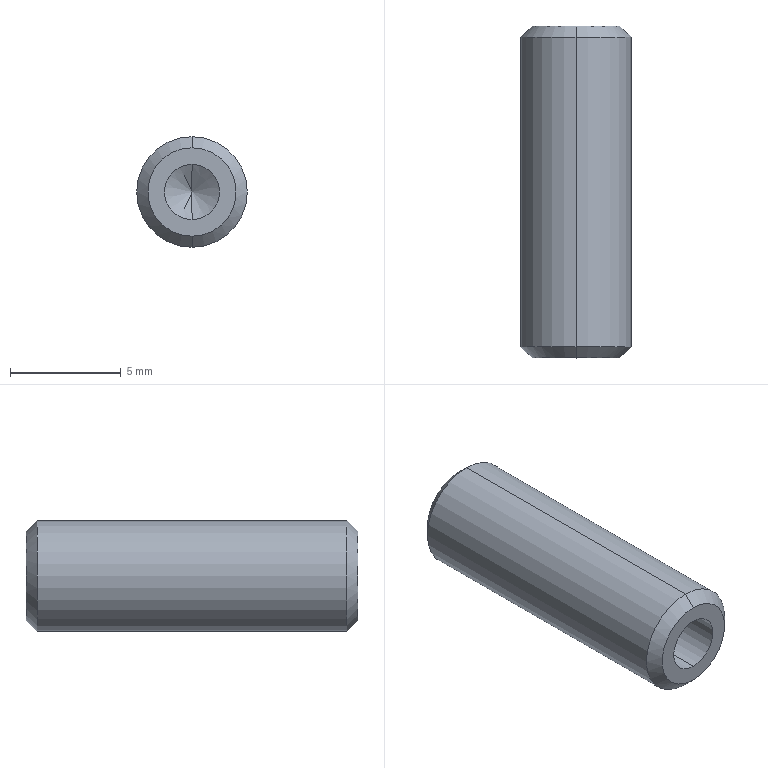Part | SolidWorks | features Chamfer 1, Extrusion 1, HoleWzd 1 | 1 solid | 12 faces | box 5 x 15 x 5 mm | volume 252.815 mm3 | cone 6 | cylinder 4 | plane 2 | commonest cylinder face diameters 2.5 x2 5 x2
STEP:
#1=CARTESIAN_POINT('',(0.,15.,2.));
#2=VERTEX_POINT('',#1);
#3=CARTESIAN_POINT('',(0.,15.,-2.));
#4=VERTEX_POINT('',#3);
#5=CARTESIAN_POINT('',(0.,15.,0.));
#6=DIRECTION('',(0.,1.,0.));
#7=DIRECTION('',(0.,0.,1.));
#8=AXIS2_PLACEMENT_3D('',#5,#6,#7);
#9=CIRCLE('',#8,2.);
#10=EDGE_CURVE('',#2,#4,#9,.T.);
#11=ORIENTED_EDGE('',*,*,#10,.F.);
#12=CARTESIAN_POINT('',(0.,14.5,2.5));
#13=VERTEX_POINT('',#12);
#14=CARTESIAN_POINT('',(0.,15.,2.));
#15=DIRECTION('',(0.,-0.7071,0.7071));
#16=VECTOR('',#15,1000.);
#17=LINE('',#14,#16);
#18=EDGE_CURVE('',#2,#13,#17,.T.);
#19=ORIENTED_EDGE('',*,*,#18,.T.);
#20=CARTESIAN_POINT('',(0.,14.5,-2.5));
#21=VERTEX_POINT('',#20);
#22=CARTESIAN_POINT('',(0.,14.5,0.));
#23=DIRECTION('',(0.,-1.,0.));
#24=DIRECTION('',(0.,0.,1.));
#25=AXIS2_PLACEMENT_3D('',#22,#23,#24);
#26=CIRCLE('',#25,2.5);
#27=EDGE_CURVE('',#21,#13,#26,.T.);
#28=ORIENTED_EDGE('',*,*,#27,.F.);
#29=CARTESIAN_POINT('',(0.,15.,-2.));
#30=DIRECTION('',(0.,-0.7071,-0.7071));
#31=VECTOR('',#30,1000.);
#32=LINE('',#29,#31);
#33=EDGE_CURVE('',#4,#21,#32,.T.);
#34=ORIENTED_EDGE('',*,*,#33,.F.);
#35=EDGE_LOOP('',(#11,#19,#28,#34));
#36=FACE_OUTER_BOUND('',#35,.T.);
#37=CARTESIAN_POINT('',(0.,15.,0.));
#38=DIRECTION('',(0.,-1.,0.));
#39=DIRECTION('',(0.,0.,-1.));
#40=AXIS2_PLACEMENT_3D('',#37,#38,#39);
#41=CONICAL_SURFACE('',#40,2.,0.7854);
#42=ADVANCED_FACE('',(#36),#41,.T.);
#43=CARTESIAN_POINT('',(0.,0.,-2.));
#44=VERTEX_POINT('',#43);
#45=CARTESIAN_POINT('',(0.,0.,2.));
#46=VERTEX_POINT('',#45);
#47=CARTESIAN_POINT('',(0.,0.,0.));
#48=DIRECTION('',(0.,-1.,0.));
#49=DIRECTION('',(0.,0.,1.));
#50=AXIS2_PLACEMENT_3D('',#47,#48,#49);
#51=CIRCLE('',#50,2.);
#52=EDGE_CURVE('',#44,#46,#51,.T.);
#53=ORIENTED_EDGE('',*,*,#52,.F.);
#54=CARTESIAN_POINT('',(0.,0.5,-2.5));
#55=VERTEX_POINT('',#54);
#56=CARTESIAN_POINT('',(0.,0.5,-2.5));
#57=DIRECTION('',(0.,0.7071,-0.7071));
#58=VECTOR('',#57,1000.);
#59=LINE('',#56,#58);
#60=EDGE_CURVE('',#44,#55,#59,.T.);
#61=ORIENTED_EDGE('',*,*,#60,.T.);
#62=CARTESIAN_POINT('',(0.,0.5,2.5));
#63=VERTEX_POINT('',#62);
#64=CARTESIAN_POINT('',(0.,0.5,0.));
#65=DIRECTION('',(0.,1.,0.));
#66=DIRECTION('',(0.,0.,1.));
#67=AXIS2_PLACEMENT_3D('',#64,#65,#66);
#68=CIRCLE('',#67,2.5);
#69=EDGE_CURVE('',#63,#55,#68,.T.);
#70=ORIENTED_EDGE('',*,*,#69,.F.);
#71=CARTESIAN_POINT('',(0.,0.5,2.5));
#72=DIRECTION('',(0.,0.7071,0.7071));
#73=VECTOR('',#72,1000.);
#74=LINE('',#71,#73);
#75=EDGE_CURVE('',#46,#63,#74,.T.);
#76=ORIENTED_EDGE('',*,*,#75,.F.);
#77=EDGE_LOOP('',(#53,#61,#70,#76));
#78=FACE_OUTER_BOUND('',#77,.T.);
#79=CARTESIAN_POINT('',(0.,0.5,0.));
#80=DIRECTION('',(0.,1.,0.));
#81=DIRECTION('',(0.,0.,1.));
#82=AXIS2_PLACEMENT_3D('',#79,#80,#81);
#83=CONICAL_SURFACE('',#82,2.5,0.7854);
#84=ADVANCED_FACE('',(#78),#83,.T.);
#85=CARTESIAN_POINT('',(0.,7.5,1.25));
#86=VERTEX_POINT('',#85);
#87=CARTESIAN_POINT('',(0.,7.5,-1.25));
#88=VERTEX_POINT('',#87);
#89=CARTESIAN_POINT('',(0.,7.5,0.));
#90=DIRECTION('',(0.,-1.,0.));
#91=DIRECTION('',(0.,0.,-1.));
#92=AXIS2_PLACEMENT_3D('',#89,#90,#91);
#93=CIRCLE('',#92,1.25);
#94=EDGE_CURVE('',#86,#88,#93,.T.);
#95=ORIENTED_EDGE('',*,*,#94,.F.);
#96=CARTESIAN_POINT('',(0.,0.,1.25));
#97=VERTEX_POINT('',#96);
#98=CARTESIAN_POINT('',(0.,0.,1.25));
#99=DIRECTION('',(0.,-1.,0.));
#100=VECTOR('',#99,1000.);
#101=LINE('',#98,#100);
#102=EDGE_CURVE('',#86,#97,#101,.T.);
#103=ORIENTED_EDGE('',*,*,#102,.T.);
#104=CARTESIAN_POINT('',(0.,0.,-1.25));
#105=VERTEX_POINT('',#104);
#106=CARTESIAN_POINT('',(0.,0.,0.));
#107=DIRECTION('',(0.,-1.,0.));
#108=DIRECTION('',(0.,0.,-1.));
#109=AXIS2_PLACEMENT_3D('',#106,#107,#108);
#110=CIRCLE('',#109,1.25);
#111=EDGE_CURVE('',#97,#105,#110,.T.);
#112=ORIENTED_EDGE('',*,*,#111,.T.);
#113=CARTESIAN_POINT('',(0.,0.,-1.25));
#114=DIRECTION('',(0.,-1.,0.));
#115=VECTOR('',#114,1000.);
#116=LINE('',#113,#115);
#117=EDGE_CURVE('',#88,#105,#116,.T.);
#118=ORIENTED_EDGE('',*,*,#117,.F.);
#119=EDGE_LOOP('',(#95,#103,#112,#118));
#120=FACE_OUTER_BOUND('',#119,.T.);
#121=CARTESIAN_POINT('',(0.,0.,0.));
#122=DIRECTION('',(0.,-1.,0.));
#123=DIRECTION('',(0.,0.,-1.));
#124=AXIS2_PLACEMENT_3D('',#121,#122,#123);
#125=CYLINDRICAL_SURFACE('',#124,1.25);
#126=ADVANCED_FACE('',(#120),#125,.F.);
#127=CARTESIAN_POINT('',(0.,8.251,0.));
#128=VERTEX_POINT('',#127);
#129=CARTESIAN_POINT('',(0.,7.5,-1.25));
#130=DIRECTION('',(0.,-0.515,-0.8572));
#131=VECTOR('',#130,1000.);
#132=LINE('',#129,#131);
#133=EDGE_CURVE('',#128,#88,#132,.T.);
#134=ORIENTED_EDGE('',*,*,#133,.F.);
#135=CARTESIAN_POINT('',(0.,7.5,1.25));
#136=DIRECTION('',(0.,-0.515,0.8572));
#137=VECTOR('',#136,1000.);
#138=LINE('',#135,#137);
#139=EDGE_CURVE('',#128,#86,#138,.T.);
#140=ORIENTED_EDGE('',*,*,#139,.T.);
#141=ORIENTED_EDGE('',*,*,#94,.T.);
#142=EDGE_LOOP('',(#134,#140,#141));
#143=FACE_OUTER_BOUND('',#142,.T.);
#144=CARTESIAN_POINT('',(0.,7.5,0.));
#145=DIRECTION('',(0.,-1.,0.));
#146=DIRECTION('',(0.,0.,-1.));
#147=AXIS2_PLACEMENT_3D('',#144,#145,#146);
#148=CONICAL_SURFACE('',#147,1.25,1.03);
#149=ADVANCED_FACE('',(#143),#148,.F.);
#150=ORIENTED_EDGE('',*,*,#27,.T.);
#151=CARTESIAN_POINT('',(0.,15.,2.5));
#152=DIRECTION('',(0.,-1.,0.));
#153=VECTOR('',#152,1000.);
#154=LINE('',#151,#153);
#155=EDGE_CURVE('',#13,#63,#154,.T.);
#156=ORIENTED_EDGE('',*,*,#155,.T.);
#157=ORIENTED_EDGE('',*,*,#69,.T.);
#158=CARTESIAN_POINT('',(0.,15.,-2.5));
#159=DIRECTION('',(0.,-1.,0.));
#160=VECTOR('',#159,1000.);
#161=LINE('',#158,#160);
#162=EDGE_CURVE('',#21,#55,#161,.T.);
#163=ORIENTED_EDGE('',*,*,#162,.F.);
#164=EDGE_LOOP('',(#150,#156,#157,#163));
#165=FACE_OUTER_BOUND('',#164,.T.);
#166=CARTESIAN_POINT('',(0.,15.,0.));
#167=DIRECTION('',(0.,-1.,0.));
#168=DIRECTION('',(0.,0.,-1.));
#169=AXIS2_PLACEMENT_3D('',#166,#167,#168);
#170=CYLINDRICAL_SURFACE('',#169,2.5);
#171=ADVANCED_FACE('',(#165),#170,.T.);
#172=ORIENTED_EDGE('',*,*,#155,.F.);
#173=CARTESIAN_POINT('',(0.,14.5,0.));
#174=DIRECTION('',(0.,-1.,0.));
#175=DIRECTION('',(0.,0.,1.));
#176=AXIS2_PLACEMENT_3D('',#173,#174,#175);
#177=CIRCLE('',#176,2.5);
#178=EDGE_CURVE('',#13,#21,#177,.T.);
#179=ORIENTED_EDGE('',*,*,#178,.T.);
#180=ORIENTED_EDGE('',*,*,#162,.T.);
#181=CARTESIAN_POINT('',(0.,0.5,0.));
#182=DIRECTION('',(0.,1.,0.));
#183=DIRECTION('',(0.,0.,1.));
#184=AXIS2_PLACEMENT_3D('',#181,#182,#183);
#185=CIRCLE('',#184,2.5);
#186=EDGE_CURVE('',#55,#63,#185,.T.);
#187=ORIENTED_EDGE('',*,*,#186,.T.);
#188=EDGE_LOOP('',(#172,#179,#180,#187));
#189=FACE_OUTER_BOUND('',#188,.T.);
#190=CARTESIAN_POINT('',(0.,15.,0.));
#191=DIRECTION('',(0.,-1.,0.));
#192=DIRECTION('',(0.,0.,-1.));
#193=AXIS2_PLACEMENT_3D('',#190,#191,#192);
#194=CYLINDRICAL_SURFACE('',#193,2.5);
#195=ADVANCED_FACE('',(#189),#194,.T.);
#196=CARTESIAN_POINT('',(0.,15.,0.));
#197=DIRECTION('',(0.,1.,0.));
#198=DIRECTION('',(0.,0.,1.));
#199=AXIS2_PLACEMENT_3D('',#196,#197,#198);
#200=CIRCLE('',#199,2.);
#201=EDGE_CURVE('',#4,#2,#200,.T.);
#202=ORIENTED_EDGE('',*,*,#201,.T.);
#203=ORIENTED_EDGE('',*,*,#10,.T.);
#204=EDGE_LOOP('',(#202,#203));
#205=FACE_OUTER_BOUND('',#204,.T.);
#206=CARTESIAN_POINT('',(0.,15.,0.));
#207=DIRECTION('',(0.,1.,0.));
#208=DIRECTION('',(0.,0.,1.));
#209=AXIS2_PLACEMENT_3D('',#206,#207,#208);
#210=PLANE('',#209);
#211=ADVANCED_FACE('',(#205),#210,.T.);
#212=CARTESIAN_POINT('',(0.,0.,0.));
#213=DIRECTION('',(0.,-1.,0.));
#214=DIRECTION('',(0.,0.,1.));
#215=AXIS2_PLACEMENT_3D('',#212,#213,#214);
#216=CIRCLE('',#215,2.);
#217=EDGE_CURVE('',#46,#44,#216,.T.);
#218=ORIENTED_EDGE('',*,*,#217,.T.);
#219=ORIENTED_EDGE('',*,*,#52,.T.);
#220=EDGE_LOOP('',(#218,#219));
#221=FACE_OUTER_BOUND('',#220,.T.);
#222=CARTESIAN_POINT('',(0.,0.,0.));
#223=DIRECTION('',(0.,-1.,0.));
#224=DIRECTION('',(0.,0.,-1.));
#225=AXIS2_PLACEMENT_3D('',#222,#223,#224);
#226=CIRCLE('',#225,1.25);
#227=EDGE_CURVE('',#105,#97,#226,.T.);
#228=ORIENTED_EDGE('',*,*,#227,.F.);
#229=ORIENTED_EDGE('',*,*,#111,.F.);
#230=EDGE_LOOP('',(#228,#229));
#231=FACE_BOUND('',#230,.T.);
#232=CARTESIAN_POINT('',(0.,0.,0.));
#233=DIRECTION('',(0.,1.,0.));
#234=DIRECTION('',(0.,0.,1.));
#235=AXIS2_PLACEMENT_3D('',#232,#233,#234);
#236=PLANE('',#235);
#237=ADVANCED_FACE('',(#221,#231),#236,.F.);
#238=ORIENTED_EDGE('',*,*,#139,.F.);
#239=ORIENTED_EDGE('',*,*,#133,.T.);
#240=CARTESIAN_POINT('',(0.,7.5,0.));
#241=DIRECTION('',(0.,-1.,0.));
#242=DIRECTION('',(0.,0.,-1.));
#243=AXIS2_PLACEMENT_3D('',#240,#241,#242);
#244=CIRCLE('',#243,1.25);
#245=EDGE_CURVE('',#88,#86,#244,.T.);
#246=ORIENTED_EDGE('',*,*,#245,.T.);
#247=EDGE_LOOP('',(#238,#239,#246));
#248=FACE_OUTER_BOUND('',#247,.T.);
#249=CARTESIAN_POINT('',(0.,7.5,0.));
#250=DIRECTION('',(0.,-1.,0.));
#251=DIRECTION('',(0.,0.,-1.));
#252=AXIS2_PLACEMENT_3D('',#249,#250,#251);
#253=CONICAL_SURFACE('',#252,1.25,1.03);
#254=ADVANCED_FACE('',(#248),#253,.F.);
#255=ORIENTED_EDGE('',*,*,#102,.F.);
#256=ORIENTED_EDGE('',*,*,#245,.F.);
#257=ORIENTED_EDGE('',*,*,#117,.T.);
#258=ORIENTED_EDGE('',*,*,#227,.T.);
#259=EDGE_LOOP('',(#255,#256,#257,#258));
#260=FACE_OUTER_BOUND('',#259,.T.);
#261=CARTESIAN_POINT('',(0.,0.,0.));
#262=DIRECTION('',(0.,-1.,0.));
#263=DIRECTION('',(0.,0.,-1.));
#264=AXIS2_PLACEMENT_3D('',#261,#262,#263);
#265=CYLINDRICAL_SURFACE('',#264,1.25);
#266=ADVANCED_FACE('',(#260),#265,.F.);
#267=ORIENTED_EDGE('',*,*,#60,.F.);
#268=ORIENTED_EDGE('',*,*,#217,.F.);
#269=ORIENTED_EDGE('',*,*,#75,.T.);
#270=ORIENTED_EDGE('',*,*,#186,.F.);
#271=EDGE_LOOP('',(#267,#268,#269,#270));
#272=FACE_OUTER_BOUND('',#271,.T.);
#273=CARTESIAN_POINT('',(0.,0.5,0.));
#274=DIRECTION('',(0.,1.,0.));
#275=DIRECTION('',(0.,0.,1.));
#276=AXIS2_PLACEMENT_3D('',#273,#274,#275);
#277=CONICAL_SURFACE('',#276,2.5,0.7854);
#278=ADVANCED_FACE('',(#272),#277,.T.);
#279=ORIENTED_EDGE('',*,*,#18,.F.);
#280=ORIENTED_EDGE('',*,*,#201,.F.);
#281=ORIENTED_EDGE('',*,*,#33,.T.);
#282=ORIENTED_EDGE('',*,*,#178,.F.);
#283=EDGE_LOOP('',(#279,#280,#281,#282));
#284=FACE_OUTER_BOUND('',#283,.T.);
#285=CARTESIAN_POINT('',(0.,15.,0.));
#286=DIRECTION('',(0.,-1.,0.));
#287=DIRECTION('',(0.,0.,-1.));
#288=AXIS2_PLACEMENT_3D('',#285,#286,#287);
#289=CONICAL_SURFACE('',#288,2.,0.7854);
#290=ADVANCED_FACE('',(#284),#289,.T.);
#291=CLOSED_SHELL('',(#42,#84,#126,#149,#171,#195,#211,#237,#254,#266,#278,#290));
#292=MANIFOLD_SOLID_BREP('',#291);
#293=CARTESIAN_POINT('',(0.,0.,0.));
#294=DIRECTION('',(0.,0.,1.));
#295=DIRECTION('',(1.,0.,0.));
#296=AXIS2_PLACEMENT_3D('',#293,#294,#295);
#297=(LENGTH_UNIT()NAMED_UNIT(*)SI_UNIT(.MILLI.,.METRE.));
#298=UNCERTAINTY_MEASURE_WITH_UNIT(LENGTH_MEASURE(0.00001),#297,'','');
#299=(NAMED_UNIT(*)PLANE_ANGLE_UNIT()SI_UNIT($,.RADIAN.));
#300=(NAMED_UNIT(*)SI_UNIT($,.STERADIAN.)SOLID_ANGLE_UNIT());
#301=(GEOMETRIC_REPRESENTATION_CONTEXT(3)GLOBAL_UNCERTAINTY_ASSIGNED_CONTEXT((#298))GLOBAL_UNIT_ASSIGNED_CONTEXT((#297,#299,#300))REPRESENTATION_CONTEXT('',''));
#302=ADVANCED_BREP_SHAPE_REPRESENTATION('',(#292,#296),#301);